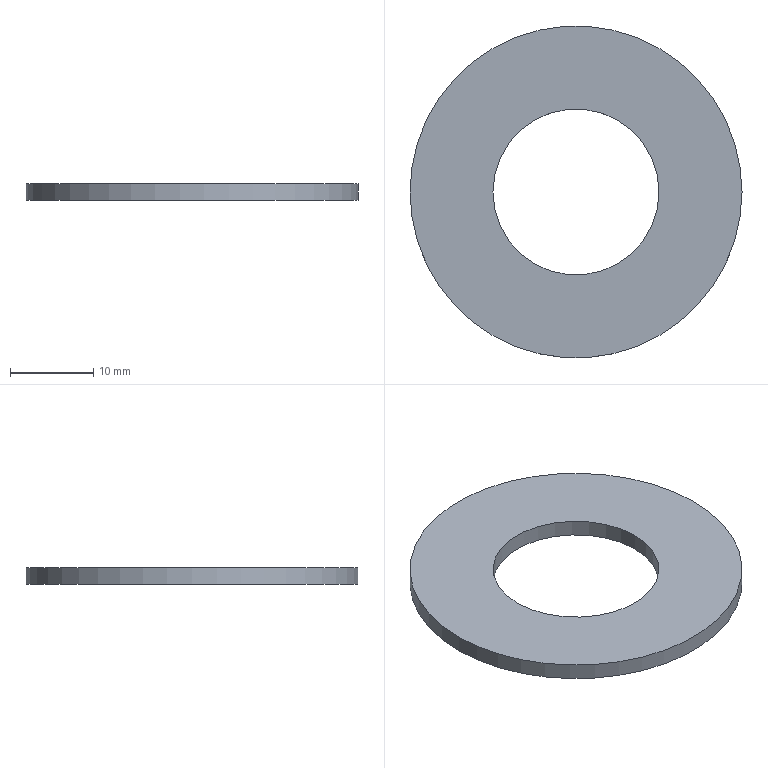Part | NX | features DATUM_CSYS 2, EXTRUDE 1, SKETCH 1 | 1 solid | 4 faces | box 40 x 40 x 2 mm | volume 1885 mm3 | cylinder 2 | plane 2 | commonest cylinder face diameters 20 x1 40 x1
STEP:
#1=CARTESIAN_POINT('',(20.,0.,2.));
#2=VERTEX_POINT('',#1);
#3=CARTESIAN_POINT('',(0.,0.,2.));
#4=DIRECTION('',(0.,0.,1.));
#5=DIRECTION('',(1.,0.,0.));
#6=AXIS2_PLACEMENT_3D('',#3,#4,#5);
#7=CIRCLE('',#6,20.);
#8=EDGE_CURVE('',#2,#2,#7,.T.);
#9=ORIENTED_EDGE('',*,*,#8,.F.);
#10=EDGE_LOOP('',(#9));
#11=FACE_BOUND('',#10,.T.);
#12=CARTESIAN_POINT('',(20.,0.,0.));
#13=VERTEX_POINT('',#12);
#14=CARTESIAN_POINT('',(0.,0.,0.));
#15=DIRECTION('',(0.,0.,1.));
#16=DIRECTION('',(1.,0.,0.));
#17=AXIS2_PLACEMENT_3D('',#14,#15,#16);
#18=CIRCLE('',#17,20.);
#19=EDGE_CURVE('',#13,#13,#18,.T.);
#20=ORIENTED_EDGE('',*,*,#19,.T.);
#21=EDGE_LOOP('',(#20));
#22=FACE_BOUND('',#21,.T.);
#23=CARTESIAN_POINT('',(0.,0.,2.));
#24=DIRECTION('',(0.,0.,-1.));
#25=DIRECTION('',(-1.,0.,0.));
#26=AXIS2_PLACEMENT_3D('',#23,#24,#25);
#27=CYLINDRICAL_SURFACE('',#26,20.);
#28=ADVANCED_FACE('',(#11,#22),#27,.T.);
#29=CARTESIAN_POINT('',(10.,0.,2.));
#30=VERTEX_POINT('',#29);
#31=CARTESIAN_POINT('',(0.,0.,2.));
#32=DIRECTION('',(0.,0.,1.));
#33=DIRECTION('',(1.,0.,0.));
#34=AXIS2_PLACEMENT_3D('',#31,#32,#33);
#35=CIRCLE('',#34,10.);
#36=EDGE_CURVE('',#30,#30,#35,.T.);
#37=ORIENTED_EDGE('',*,*,#36,.T.);
#38=EDGE_LOOP('',(#37));
#39=FACE_BOUND('',#38,.T.);
#40=CARTESIAN_POINT('',(10.,0.,0.));
#41=VERTEX_POINT('',#40);
#42=CARTESIAN_POINT('',(0.,0.,0.));
#43=DIRECTION('',(0.,0.,1.));
#44=DIRECTION('',(1.,0.,0.));
#45=AXIS2_PLACEMENT_3D('',#42,#43,#44);
#46=CIRCLE('',#45,10.);
#47=EDGE_CURVE('',#41,#41,#46,.T.);
#48=ORIENTED_EDGE('',*,*,#47,.F.);
#49=EDGE_LOOP('',(#48));
#50=FACE_BOUND('',#49,.T.);
#51=CARTESIAN_POINT('',(0.,0.,2.));
#52=DIRECTION('',(0.,0.,-1.));
#53=DIRECTION('',(-1.,0.,0.));
#54=AXIS2_PLACEMENT_3D('',#51,#52,#53);
#55=CYLINDRICAL_SURFACE('',#54,10.);
#56=ADVANCED_FACE('',(#39,#50),#55,.F.);
#57=ORIENTED_EDGE('',*,*,#8,.T.);
#58=EDGE_LOOP('',(#57));
#59=FACE_BOUND('',#58,.T.);
#60=ORIENTED_EDGE('',*,*,#36,.F.);
#61=EDGE_LOOP('',(#60));
#62=FACE_BOUND('',#61,.T.);
#63=CARTESIAN_POINT('',(0.,0.,2.));
#64=DIRECTION('',(0.,0.,1.));
#65=DIRECTION('',(1.,0.,0.));
#66=AXIS2_PLACEMENT_3D('',#63,#64,#65);
#67=PLANE('',#66);
#68=ADVANCED_FACE('',(#59,#62),#67,.T.);
#69=ORIENTED_EDGE('',*,*,#19,.F.);
#70=EDGE_LOOP('',(#69));
#71=FACE_BOUND('',#70,.T.);
#72=ORIENTED_EDGE('',*,*,#47,.T.);
#73=EDGE_LOOP('',(#72));
#74=FACE_BOUND('',#73,.T.);
#75=CARTESIAN_POINT('',(0.,0.,0.));
#76=DIRECTION('',(0.,0.,1.));
#77=DIRECTION('',(1.,0.,0.));
#78=AXIS2_PLACEMENT_3D('',#75,#76,#77);
#79=PLANE('',#78);
#80=ADVANCED_FACE('',(#71,#74),#79,.F.);
#81=CLOSED_SHELL('',(#28,#56,#68,#80));
#82=MANIFOLD_SOLID_BREP('',#81);
#83=(LENGTH_UNIT()NAMED_UNIT(*)SI_UNIT(.MILLI.,.METRE.));
#84=UNCERTAINTY_MEASURE_WITH_UNIT(LENGTH_MEASURE(0.00001),#83,'','');
#85=(NAMED_UNIT(*)PLANE_ANGLE_UNIT()SI_UNIT($,.RADIAN.));
#86=(NAMED_UNIT(*)SI_UNIT($,.STERADIAN.)SOLID_ANGLE_UNIT());
#87=(GEOMETRIC_REPRESENTATION_CONTEXT(3)GLOBAL_UNCERTAINTY_ASSIGNED_CONTEXT((#84))GLOBAL_UNIT_ASSIGNED_CONTEXT((#83,#85,#86))REPRESENTATION_CONTEXT('',''));
#88=ADVANCED_BREP_SHAPE_REPRESENTATION('',(#82),#87);